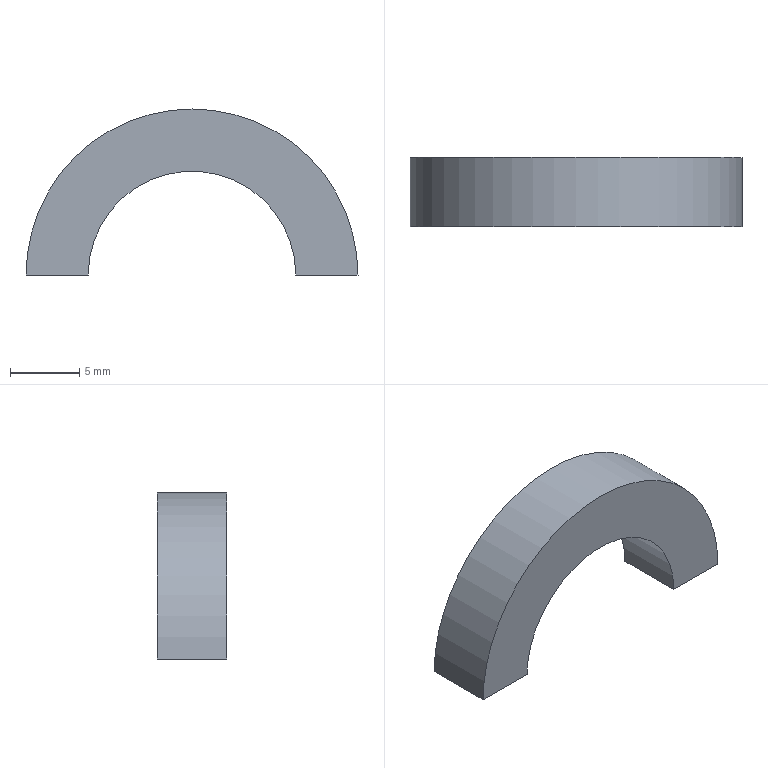Part | STEP file | 6802 ZZ | 1 solid | 6 faces | box 24 x 5 x 12 mm | volume 689.187 mm3 | plane 4 | cylinder 2 | commonest cylinder face diameters 15 x1 24 x1
STEP:
#1=CARTESIAN_POINT('',(0.,0.,0.));
#2=DIRECTION('',(0.,0.,1.));
#3=DIRECTION('',(1.,0.,0.));
#4=AXIS2_PLACEMENT_3D('',#1,#2,#3);
#5=CARTESIAN_POINT('',(-12.,5.,0.));
#6=VERTEX_POINT('',#5);
#7=CARTESIAN_POINT('',(-7.5,5.,0.));
#8=VERTEX_POINT('',#7);
#9=CARTESIAN_POINT('',(0.,5.,0.));
#10=DIRECTION('',(1.,0.,0.));
#11=VECTOR('',#10,1.);
#12=LINE('',#9,#11);
#13=CARTESIAN_POINT('',(0.,5.,0.));
#14=DIRECTION('',(0.,1.,0.));
#15=DIRECTION('',(0.,0.,1.));
#16=AXIS2_PLACEMENT_3D('',#13,#14,#15);
#17=PLANE('',#16);
#18=CARTESIAN_POINT('',(0.,0.));
#19=DIRECTION('',(0.,1.));
#20=VECTOR('',#19,1.);
#21=LINE('',#18,#20);
#22=(GEOMETRIC_REPRESENTATION_CONTEXT(2)PARAMETRIC_REPRESENTATION_CONTEXT()REPRESENTATION_CONTEXT('',''));
#23=DEFINITIONAL_REPRESENTATION('',(#21),#22);
#24=PCURVE('',#17,#23);
#25=CARTESIAN_POINT('',(60.,-35.57,0.));
#26=DIRECTION('',(0.,0.,1.));
#27=DIRECTION('',(1.,0.,0.));
#28=AXIS2_PLACEMENT_3D('',#25,#26,#27);
#29=PLANE('',#28);
#30=CARTESIAN_POINT('',(-60.,40.57));
#31=DIRECTION('',(1.,0.));
#32=VECTOR('',#31,1.);
#33=LINE('',#30,#32);
#34=(GEOMETRIC_REPRESENTATION_CONTEXT(2)PARAMETRIC_REPRESENTATION_CONTEXT()REPRESENTATION_CONTEXT('',''));
#35=DEFINITIONAL_REPRESENTATION('',(#33),#34);
#36=PCURVE('',#29,#35);
#37=SURFACE_CURVE('',#12,(#24,#36),.PCURVE_S1.);
#38=EDGE_CURVE('',#6,#8,#37,.T.);
#39=ORIENTED_EDGE('',*,*,#38,.F.);
#40=CARTESIAN_POINT('',(12.,5.,0.));
#41=VERTEX_POINT('',#40);
#42=CARTESIAN_POINT('',(0.,5.,0.));
#43=DIRECTION('',(0.,1.,0.));
#44=DIRECTION('',(0.,0.,1.));
#45=AXIS2_PLACEMENT_3D('',#42,#43,#44);
#46=CIRCLE('',#45,12.);
#47=CARTESIAN_POINT('',(0.,0.));
#48=DIRECTION('',(1.,0.));
#49=AXIS2_PLACEMENT_2D('',#47,#48);
#50=CIRCLE('',#49,12.);
#51=(GEOMETRIC_REPRESENTATION_CONTEXT(2)PARAMETRIC_REPRESENTATION_CONTEXT()REPRESENTATION_CONTEXT('',''));
#52=DEFINITIONAL_REPRESENTATION('',(#50),#51);
#53=PCURVE('',#17,#52);
#54=CARTESIAN_POINT('',(0.,5.,0.));
#55=DIRECTION('',(0.,-1.,0.));
#56=DIRECTION('',(0.,0.,-1.));
#57=AXIS2_PLACEMENT_3D('',#54,#55,#56);
#58=CYLINDRICAL_SURFACE('',#57,12.);
#59=CARTESIAN_POINT('',(9.425,0.));
#60=DIRECTION('',(-1.,0.));
#61=VECTOR('',#60,1.);
#62=LINE('',#59,#61);
#63=(GEOMETRIC_REPRESENTATION_CONTEXT(2)PARAMETRIC_REPRESENTATION_CONTEXT()REPRESENTATION_CONTEXT('',''));
#64=DEFINITIONAL_REPRESENTATION('',(#62),#63);
#65=PCURVE('',#58,#64);
#66=SURFACE_CURVE('',#46,(#53,#65),.PCURVE_S1.);
#67=EDGE_CURVE('',#6,#41,#66,.T.);
#68=ORIENTED_EDGE('',*,*,#67,.T.);
#69=CARTESIAN_POINT('',(7.5,5.,0.));
#70=VERTEX_POINT('',#69);
#71=CARTESIAN_POINT('',(0.,5.,0.));
#72=DIRECTION('',(1.,0.,0.));
#73=VECTOR('',#72,1.);
#74=LINE('',#71,#73);
#75=CARTESIAN_POINT('',(0.,0.));
#76=DIRECTION('',(0.,1.));
#77=VECTOR('',#76,1.);
#78=LINE('',#75,#77);
#79=(GEOMETRIC_REPRESENTATION_CONTEXT(2)PARAMETRIC_REPRESENTATION_CONTEXT()REPRESENTATION_CONTEXT('',''));
#80=DEFINITIONAL_REPRESENTATION('',(#78),#79);
#81=PCURVE('',#17,#80);
#82=CARTESIAN_POINT('',(60.,-35.57,0.));
#83=DIRECTION('',(0.,0.,1.));
#84=DIRECTION('',(1.,0.,0.));
#85=AXIS2_PLACEMENT_3D('',#82,#83,#84);
#86=PLANE('',#85);
#87=CARTESIAN_POINT('',(-60.,40.57));
#88=DIRECTION('',(1.,0.));
#89=VECTOR('',#88,1.);
#90=LINE('',#87,#89);
#91=(GEOMETRIC_REPRESENTATION_CONTEXT(2)PARAMETRIC_REPRESENTATION_CONTEXT()REPRESENTATION_CONTEXT('',''));
#92=DEFINITIONAL_REPRESENTATION('',(#90),#91);
#93=PCURVE('',#86,#92);
#94=SURFACE_CURVE('',#74,(#81,#93),.PCURVE_S1.);
#95=EDGE_CURVE('',#70,#41,#94,.T.);
#96=ORIENTED_EDGE('',*,*,#95,.F.);
#97=CARTESIAN_POINT('',(0.,5.,0.));
#98=DIRECTION('',(0.,1.,0.));
#99=DIRECTION('',(0.,0.,1.));
#100=AXIS2_PLACEMENT_3D('',#97,#98,#99);
#101=CIRCLE('',#100,7.5);
#102=CARTESIAN_POINT('',(0.,0.));
#103=DIRECTION('',(1.,0.));
#104=AXIS2_PLACEMENT_2D('',#102,#103);
#105=CIRCLE('',#104,7.5);
#106=(GEOMETRIC_REPRESENTATION_CONTEXT(2)PARAMETRIC_REPRESENTATION_CONTEXT()REPRESENTATION_CONTEXT('',''));
#107=DEFINITIONAL_REPRESENTATION('',(#105),#106);
#108=PCURVE('',#17,#107);
#109=CARTESIAN_POINT('',(0.,5.,0.));
#110=DIRECTION('',(0.,-1.,0.));
#111=DIRECTION('',(0.,0.,-1.));
#112=AXIS2_PLACEMENT_3D('',#109,#110,#111);
#113=CYLINDRICAL_SURFACE('',#112,7.5);
#114=CARTESIAN_POINT('',(9.425,0.));
#115=DIRECTION('',(-1.,0.));
#116=VECTOR('',#115,1.);
#117=LINE('',#114,#116);
#118=(GEOMETRIC_REPRESENTATION_CONTEXT(2)PARAMETRIC_REPRESENTATION_CONTEXT()REPRESENTATION_CONTEXT('',''));
#119=DEFINITIONAL_REPRESENTATION('',(#117),#118);
#120=PCURVE('',#113,#119);
#121=SURFACE_CURVE('',#101,(#108,#120),.PCURVE_S1.);
#122=EDGE_CURVE('',#8,#70,#121,.T.);
#123=ORIENTED_EDGE('',*,*,#122,.F.);
#124=EDGE_LOOP('',(#39,#68,#96,#123));
#125=FACE_BOUND('',#124,.T.);
#126=ADVANCED_FACE('',(#125),#17,.T.);
#127=CARTESIAN_POINT('',(-12.,0.,0.));
#128=VERTEX_POINT('',#127);
#129=CARTESIAN_POINT('',(12.,0.,0.));
#130=VERTEX_POINT('',#129);
#131=CARTESIAN_POINT('',(0.,0.,0.));
#132=DIRECTION('',(0.,1.,0.));
#133=DIRECTION('',(0.,0.,1.));
#134=AXIS2_PLACEMENT_3D('',#131,#132,#133);
#135=CIRCLE('',#134,12.);
#136=CARTESIAN_POINT('',(0.,0.,0.));
#137=DIRECTION('',(0.,1.,0.));
#138=DIRECTION('',(0.,0.,1.));
#139=AXIS2_PLACEMENT_3D('',#136,#137,#138);
#140=PLANE('',#139);
#141=CARTESIAN_POINT('',(0.,0.));
#142=DIRECTION('',(1.,0.));
#143=AXIS2_PLACEMENT_2D('',#141,#142);
#144=CIRCLE('',#143,12.);
#145=(GEOMETRIC_REPRESENTATION_CONTEXT(2)PARAMETRIC_REPRESENTATION_CONTEXT()REPRESENTATION_CONTEXT('',''));
#146=DEFINITIONAL_REPRESENTATION('',(#144),#145);
#147=PCURVE('',#140,#146);
#148=CARTESIAN_POINT('',(9.425,5.));
#149=DIRECTION('',(-1.,0.));
#150=VECTOR('',#149,1.);
#151=LINE('',#148,#150);
#152=(GEOMETRIC_REPRESENTATION_CONTEXT(2)PARAMETRIC_REPRESENTATION_CONTEXT()REPRESENTATION_CONTEXT('',''));
#153=DEFINITIONAL_REPRESENTATION('',(#151),#152);
#154=PCURVE('',#58,#153);
#155=SURFACE_CURVE('',#135,(#147,#154),.PCURVE_S1.);
#156=EDGE_CURVE('',#128,#130,#155,.T.);
#157=ORIENTED_EDGE('',*,*,#156,.F.);
#158=CARTESIAN_POINT('',(-7.5,0.,0.));
#159=VERTEX_POINT('',#158);
#160=CARTESIAN_POINT('',(0.,0.,0.));
#161=DIRECTION('',(1.,0.,0.));
#162=VECTOR('',#161,1.);
#163=LINE('',#160,#162);
#164=CARTESIAN_POINT('',(0.,0.));
#165=DIRECTION('',(0.,1.));
#166=VECTOR('',#165,1.);
#167=LINE('',#164,#166);
#168=(GEOMETRIC_REPRESENTATION_CONTEXT(2)PARAMETRIC_REPRESENTATION_CONTEXT()REPRESENTATION_CONTEXT('',''));
#169=DEFINITIONAL_REPRESENTATION('',(#167),#168);
#170=PCURVE('',#140,#169);
#171=CARTESIAN_POINT('',(-60.,35.57));
#172=DIRECTION('',(1.,0.));
#173=VECTOR('',#172,1.);
#174=LINE('',#171,#173);
#175=(GEOMETRIC_REPRESENTATION_CONTEXT(2)PARAMETRIC_REPRESENTATION_CONTEXT()REPRESENTATION_CONTEXT('',''));
#176=DEFINITIONAL_REPRESENTATION('',(#174),#175);
#177=PCURVE('',#29,#176);
#178=SURFACE_CURVE('',#163,(#170,#177),.PCURVE_S1.);
#179=EDGE_CURVE('',#128,#159,#178,.T.);
#180=ORIENTED_EDGE('',*,*,#179,.T.);
#181=CARTESIAN_POINT('',(7.5,0.,0.));
#182=VERTEX_POINT('',#181);
#183=CARTESIAN_POINT('',(0.,0.,0.));
#184=DIRECTION('',(0.,1.,0.));
#185=DIRECTION('',(0.,0.,1.));
#186=AXIS2_PLACEMENT_3D('',#183,#184,#185);
#187=CIRCLE('',#186,7.5);
#188=CARTESIAN_POINT('',(0.,0.));
#189=DIRECTION('',(1.,0.));
#190=AXIS2_PLACEMENT_2D('',#188,#189);
#191=CIRCLE('',#190,7.5);
#192=(GEOMETRIC_REPRESENTATION_CONTEXT(2)PARAMETRIC_REPRESENTATION_CONTEXT()REPRESENTATION_CONTEXT('',''));
#193=DEFINITIONAL_REPRESENTATION('',(#191),#192);
#194=PCURVE('',#140,#193);
#195=CARTESIAN_POINT('',(9.425,5.));
#196=DIRECTION('',(-1.,0.));
#197=VECTOR('',#196,1.);
#198=LINE('',#195,#197);
#199=(GEOMETRIC_REPRESENTATION_CONTEXT(2)PARAMETRIC_REPRESENTATION_CONTEXT()REPRESENTATION_CONTEXT('',''));
#200=DEFINITIONAL_REPRESENTATION('',(#198),#199);
#201=PCURVE('',#113,#200);
#202=SURFACE_CURVE('',#187,(#194,#201),.PCURVE_S1.);
#203=EDGE_CURVE('',#159,#182,#202,.T.);
#204=ORIENTED_EDGE('',*,*,#203,.T.);
#205=CARTESIAN_POINT('',(0.,0.,0.));
#206=DIRECTION('',(1.,0.,0.));
#207=VECTOR('',#206,1.);
#208=LINE('',#205,#207);
#209=CARTESIAN_POINT('',(0.,0.));
#210=DIRECTION('',(0.,1.));
#211=VECTOR('',#210,1.);
#212=LINE('',#209,#211);
#213=(GEOMETRIC_REPRESENTATION_CONTEXT(2)PARAMETRIC_REPRESENTATION_CONTEXT()REPRESENTATION_CONTEXT('',''));
#214=DEFINITIONAL_REPRESENTATION('',(#212),#213);
#215=PCURVE('',#140,#214);
#216=CARTESIAN_POINT('',(-60.,35.57));
#217=DIRECTION('',(1.,0.));
#218=VECTOR('',#217,1.);
#219=LINE('',#216,#218);
#220=(GEOMETRIC_REPRESENTATION_CONTEXT(2)PARAMETRIC_REPRESENTATION_CONTEXT()REPRESENTATION_CONTEXT('',''));
#221=DEFINITIONAL_REPRESENTATION('',(#219),#220);
#222=PCURVE('',#86,#221);
#223=SURFACE_CURVE('',#208,(#215,#222),.PCURVE_S1.);
#224=EDGE_CURVE('',#182,#130,#223,.T.);
#225=ORIENTED_EDGE('',*,*,#224,.T.);
#226=EDGE_LOOP('',(#157,#180,#204,#225));
#227=FACE_BOUND('',#226,.T.);
#228=ADVANCED_FACE('',(#227),#140,.F.);
#229=ORIENTED_EDGE('',*,*,#67,.F.);
#230=CARTESIAN_POINT('',(-12.,5.,0.));
#231=DIRECTION('',(0.,-1.,0.));
#232=VECTOR('',#231,1.);
#233=LINE('',#230,#232);
#234=CARTESIAN_POINT('',(4.712,0.));
#235=DIRECTION('',(0.,1.));
#236=VECTOR('',#235,1.);
#237=LINE('',#234,#236);
#238=(GEOMETRIC_REPRESENTATION_CONTEXT(2)PARAMETRIC_REPRESENTATION_CONTEXT()REPRESENTATION_CONTEXT('',''));
#239=DEFINITIONAL_REPRESENTATION('',(#237),#238);
#240=PCURVE('',#58,#239);
#241=CARTESIAN_POINT('',(-72.,40.57));
#242=DIRECTION('',(0.,-1.));
#243=VECTOR('',#242,1.);
#244=LINE('',#241,#243);
#245=(GEOMETRIC_REPRESENTATION_CONTEXT(2)PARAMETRIC_REPRESENTATION_CONTEXT()REPRESENTATION_CONTEXT('',''));
#246=DEFINITIONAL_REPRESENTATION('',(#244),#245);
#247=PCURVE('',#29,#246);
#248=SURFACE_CURVE('',#233,(#240,#247),.PCURVE_S1.);
#249=EDGE_CURVE('',#6,#128,#248,.T.);
#250=ORIENTED_EDGE('',*,*,#249,.T.);
#251=ORIENTED_EDGE('',*,*,#156,.T.);
#252=CARTESIAN_POINT('',(12.,5.,0.));
#253=DIRECTION('',(0.,1.,0.));
#254=VECTOR('',#253,1.);
#255=LINE('',#252,#254);
#256=CARTESIAN_POINT('',(1.571,0.));
#257=DIRECTION('',(0.,-1.));
#258=VECTOR('',#257,1.);
#259=LINE('',#256,#258);
#260=(GEOMETRIC_REPRESENTATION_CONTEXT(2)PARAMETRIC_REPRESENTATION_CONTEXT()REPRESENTATION_CONTEXT('',''));
#261=DEFINITIONAL_REPRESENTATION('',(#259),#260);
#262=PCURVE('',#58,#261);
#263=CARTESIAN_POINT('',(-48.,40.57));
#264=DIRECTION('',(0.,1.));
#265=VECTOR('',#264,1.);
#266=LINE('',#263,#265);
#267=(GEOMETRIC_REPRESENTATION_CONTEXT(2)PARAMETRIC_REPRESENTATION_CONTEXT()REPRESENTATION_CONTEXT('',''));
#268=DEFINITIONAL_REPRESENTATION('',(#266),#267);
#269=PCURVE('',#86,#268);
#270=SURFACE_CURVE('',#255,(#262,#269),.PCURVE_S1.);
#271=EDGE_CURVE('',#130,#41,#270,.T.);
#272=ORIENTED_EDGE('',*,*,#271,.T.);
#273=EDGE_LOOP('',(#229,#250,#251,#272));
#274=FACE_BOUND('',#273,.T.);
#275=ADVANCED_FACE('',(#274),#58,.T.);
#276=ORIENTED_EDGE('',*,*,#203,.T.);
#277=CARTESIAN_POINT('',(7.5,5.,0.));
#278=DIRECTION('',(0.,1.,0.));
#279=VECTOR('',#278,1.);
#280=LINE('',#277,#279);
#281=CARTESIAN_POINT('',(1.571,0.));
#282=DIRECTION('',(0.,-1.));
#283=VECTOR('',#282,1.);
#284=LINE('',#281,#283);
#285=(GEOMETRIC_REPRESENTATION_CONTEXT(2)PARAMETRIC_REPRESENTATION_CONTEXT()REPRESENTATION_CONTEXT('',''));
#286=DEFINITIONAL_REPRESENTATION('',(#284),#285);
#287=PCURVE('',#113,#286);
#288=CARTESIAN_POINT('',(-52.5,40.57));
#289=DIRECTION('',(0.,1.));
#290=VECTOR('',#289,1.);
#291=LINE('',#288,#290);
#292=(GEOMETRIC_REPRESENTATION_CONTEXT(2)PARAMETRIC_REPRESENTATION_CONTEXT()REPRESENTATION_CONTEXT('',''));
#293=DEFINITIONAL_REPRESENTATION('',(#291),#292);
#294=PCURVE('',#86,#293);
#295=SURFACE_CURVE('',#280,(#287,#294),.PCURVE_S1.);
#296=EDGE_CURVE('',#182,#70,#295,.T.);
#297=ORIENTED_EDGE('',*,*,#296,.T.);
#298=ORIENTED_EDGE('',*,*,#122,.F.);
#299=CARTESIAN_POINT('',(-7.5,5.,0.));
#300=DIRECTION('',(0.,-1.,0.));
#301=VECTOR('',#300,1.);
#302=LINE('',#299,#301);
#303=CARTESIAN_POINT('',(4.712,0.));
#304=DIRECTION('',(0.,1.));
#305=VECTOR('',#304,1.);
#306=LINE('',#303,#305);
#307=(GEOMETRIC_REPRESENTATION_CONTEXT(2)PARAMETRIC_REPRESENTATION_CONTEXT()REPRESENTATION_CONTEXT('',''));
#308=DEFINITIONAL_REPRESENTATION('',(#306),#307);
#309=PCURVE('',#113,#308);
#310=CARTESIAN_POINT('',(-67.5,40.57));
#311=DIRECTION('',(0.,-1.));
#312=VECTOR('',#311,1.);
#313=LINE('',#310,#312);
#314=(GEOMETRIC_REPRESENTATION_CONTEXT(2)PARAMETRIC_REPRESENTATION_CONTEXT()REPRESENTATION_CONTEXT('',''));
#315=DEFINITIONAL_REPRESENTATION('',(#313),#314);
#316=PCURVE('',#29,#315);
#317=SURFACE_CURVE('',#302,(#309,#316),.PCURVE_S1.);
#318=EDGE_CURVE('',#8,#159,#317,.T.);
#319=ORIENTED_EDGE('',*,*,#318,.T.);
#320=EDGE_LOOP('',(#276,#297,#298,#319));
#321=FACE_BOUND('',#320,.F.);
#322=ADVANCED_FACE('',(#321),#113,.F.);
#323=ORIENTED_EDGE('',*,*,#224,.F.);
#324=ORIENTED_EDGE('',*,*,#296,.T.);
#325=ORIENTED_EDGE('',*,*,#95,.T.);
#326=ORIENTED_EDGE('',*,*,#271,.F.);
#327=EDGE_LOOP('',(#323,#324,#325,#326));
#328=FACE_BOUND('',#327,.T.);
#329=ADVANCED_FACE('',(#328),#86,.F.);
#330=ORIENTED_EDGE('',*,*,#38,.T.);
#331=ORIENTED_EDGE('',*,*,#318,.T.);
#332=ORIENTED_EDGE('',*,*,#179,.F.);
#333=ORIENTED_EDGE('',*,*,#249,.F.);
#334=EDGE_LOOP('',(#330,#331,#332,#333));
#335=FACE_BOUND('',#334,.T.);
#336=ADVANCED_FACE('',(#335),#29,.F.);
#337=CLOSED_SHELL('',(#126,#228,#275,#322,#329,#336));
#338=MANIFOLD_SOLID_BREP('',#337);
#339=(LENGTH_UNIT()NAMED_UNIT(*)SI_UNIT(.MILLI.,.METRE.));
#340=UNCERTAINTY_MEASURE_WITH_UNIT(LENGTH_MEASURE(0.0000001),#339,'','');
#341=(NAMED_UNIT(*)PLANE_ANGLE_UNIT()SI_UNIT($,.RADIAN.));
#342=(NAMED_UNIT(*)SI_UNIT($,.STERADIAN.)SOLID_ANGLE_UNIT());
#343=(GEOMETRIC_REPRESENTATION_CONTEXT(3)GLOBAL_UNCERTAINTY_ASSIGNED_CONTEXT((#340))GLOBAL_UNIT_ASSIGNED_CONTEXT((#339,#341,#342))REPRESENTATION_CONTEXT('',''));
#344=ADVANCED_BREP_SHAPE_REPRESENTATION('',(#4,#338),#343);